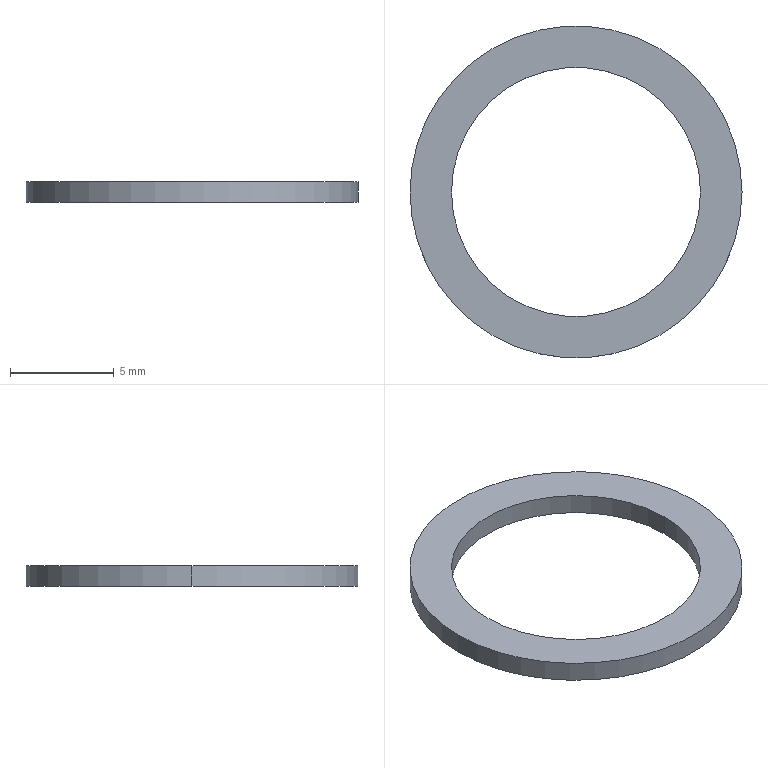Part | SolidWorks | features Extrusion 1 | 1 solid | 6 faces | box 16 x 16 x 1 mm | volume 87.965 mm3 | cylinder 4 | plane 2 | commonest cylinder face diameters 12 x2 16 x2
STEP:
#1=CARTESIAN_POINT('',(-6.,0.,1.));
#2=VERTEX_POINT('',#1);
#3=CARTESIAN_POINT('',(6.,0.,1.));
#4=VERTEX_POINT('',#3);
#5=CARTESIAN_POINT('',(0.,0.,1.));
#6=DIRECTION('',(0.,0.,1.));
#7=DIRECTION('',(1.,0.,0.));
#8=AXIS2_PLACEMENT_3D('',#5,#6,#7);
#9=CIRCLE('',#8,6.);
#10=EDGE_CURVE('',#2,#4,#9,.T.);
#11=ORIENTED_EDGE('',*,*,#10,.T.);
#12=CARTESIAN_POINT('',(6.,0.,0.));
#13=VERTEX_POINT('',#12);
#14=CARTESIAN_POINT('',(6.,0.,1.));
#15=DIRECTION('',(0.,0.,-1.));
#16=VECTOR('',#15,1000.);
#17=LINE('',#14,#16);
#18=EDGE_CURVE('',#4,#13,#17,.T.);
#19=ORIENTED_EDGE('',*,*,#18,.T.);
#20=CARTESIAN_POINT('',(-6.,0.,0.));
#21=VERTEX_POINT('',#20);
#22=CARTESIAN_POINT('',(0.,0.,0.));
#23=DIRECTION('',(0.,0.,1.));
#24=DIRECTION('',(1.,0.,0.));
#25=AXIS2_PLACEMENT_3D('',#22,#23,#24);
#26=CIRCLE('',#25,6.);
#27=EDGE_CURVE('',#21,#13,#26,.T.);
#28=ORIENTED_EDGE('',*,*,#27,.F.);
#29=CARTESIAN_POINT('',(-6.,0.,1.));
#30=DIRECTION('',(0.,0.,-1.));
#31=VECTOR('',#30,1000.);
#32=LINE('',#29,#31);
#33=EDGE_CURVE('',#2,#21,#32,.T.);
#34=ORIENTED_EDGE('',*,*,#33,.F.);
#35=EDGE_LOOP('',(#11,#19,#28,#34));
#36=FACE_OUTER_BOUND('',#35,.T.);
#37=CARTESIAN_POINT('',(0.,0.,1.));
#38=DIRECTION('',(0.,0.,-1.));
#39=DIRECTION('',(-1.,0.,0.));
#40=AXIS2_PLACEMENT_3D('',#37,#38,#39);
#41=CYLINDRICAL_SURFACE('',#40,6.);
#42=ADVANCED_FACE('',(#36),#41,.F.);
#43=CARTESIAN_POINT('',(8.,0.,1.));
#44=VERTEX_POINT('',#43);
#45=CARTESIAN_POINT('',(-8.,0.,1.));
#46=VERTEX_POINT('',#45);
#47=CARTESIAN_POINT('',(0.,0.,1.));
#48=DIRECTION('',(0.,0.,1.));
#49=DIRECTION('',(1.,0.,0.));
#50=AXIS2_PLACEMENT_3D('',#47,#48,#49);
#51=CIRCLE('',#50,8.);
#52=EDGE_CURVE('',#44,#46,#51,.T.);
#53=ORIENTED_EDGE('',*,*,#52,.F.);
#54=CARTESIAN_POINT('',(8.,0.,0.));
#55=VERTEX_POINT('',#54);
#56=CARTESIAN_POINT('',(8.,0.,1.));
#57=DIRECTION('',(0.,0.,-1.));
#58=VECTOR('',#57,1000.);
#59=LINE('',#56,#58);
#60=EDGE_CURVE('',#44,#55,#59,.T.);
#61=ORIENTED_EDGE('',*,*,#60,.T.);
#62=CARTESIAN_POINT('',(-8.,0.,0.));
#63=VERTEX_POINT('',#62);
#64=CARTESIAN_POINT('',(0.,0.,0.));
#65=DIRECTION('',(0.,0.,1.));
#66=DIRECTION('',(1.,0.,0.));
#67=AXIS2_PLACEMENT_3D('',#64,#65,#66);
#68=CIRCLE('',#67,8.);
#69=EDGE_CURVE('',#55,#63,#68,.T.);
#70=ORIENTED_EDGE('',*,*,#69,.T.);
#71=CARTESIAN_POINT('',(-8.,0.,1.));
#72=DIRECTION('',(0.,0.,-1.));
#73=VECTOR('',#72,1000.);
#74=LINE('',#71,#73);
#75=EDGE_CURVE('',#46,#63,#74,.T.);
#76=ORIENTED_EDGE('',*,*,#75,.F.);
#77=EDGE_LOOP('',(#53,#61,#70,#76));
#78=FACE_OUTER_BOUND('',#77,.T.);
#79=CARTESIAN_POINT('',(0.,0.,1.));
#80=DIRECTION('',(0.,0.,-1.));
#81=DIRECTION('',(-1.,0.,0.));
#82=AXIS2_PLACEMENT_3D('',#79,#80,#81);
#83=CYLINDRICAL_SURFACE('',#82,8.);
#84=ADVANCED_FACE('',(#78),#83,.T.);
#85=CARTESIAN_POINT('',(0.,0.,1.));
#86=DIRECTION('',(0.,0.,1.));
#87=DIRECTION('',(1.,0.,0.));
#88=AXIS2_PLACEMENT_3D('',#85,#86,#87);
#89=CIRCLE('',#88,8.);
#90=EDGE_CURVE('',#46,#44,#89,.T.);
#91=ORIENTED_EDGE('',*,*,#90,.T.);
#92=ORIENTED_EDGE('',*,*,#52,.T.);
#93=EDGE_LOOP('',(#91,#92));
#94=FACE_OUTER_BOUND('',#93,.T.);
#95=ORIENTED_EDGE('',*,*,#10,.F.);
#96=CARTESIAN_POINT('',(0.,0.,1.));
#97=DIRECTION('',(0.,0.,1.));
#98=DIRECTION('',(1.,0.,0.));
#99=AXIS2_PLACEMENT_3D('',#96,#97,#98);
#100=CIRCLE('',#99,6.);
#101=EDGE_CURVE('',#4,#2,#100,.T.);
#102=ORIENTED_EDGE('',*,*,#101,.F.);
#103=EDGE_LOOP('',(#95,#102));
#104=FACE_BOUND('',#103,.T.);
#105=CARTESIAN_POINT('',(0.,0.,1.));
#106=DIRECTION('',(0.,0.,1.));
#107=DIRECTION('',(1.,0.,0.));
#108=AXIS2_PLACEMENT_3D('',#105,#106,#107);
#109=PLANE('',#108);
#110=ADVANCED_FACE('',(#94,#104),#109,.T.);
#111=CARTESIAN_POINT('',(0.,0.,0.));
#112=DIRECTION('',(0.,0.,1.));
#113=DIRECTION('',(1.,0.,0.));
#114=AXIS2_PLACEMENT_3D('',#111,#112,#113);
#115=CIRCLE('',#114,8.);
#116=EDGE_CURVE('',#63,#55,#115,.T.);
#117=ORIENTED_EDGE('',*,*,#116,.F.);
#118=ORIENTED_EDGE('',*,*,#69,.F.);
#119=EDGE_LOOP('',(#117,#118));
#120=FACE_OUTER_BOUND('',#119,.T.);
#121=ORIENTED_EDGE('',*,*,#27,.T.);
#122=CARTESIAN_POINT('',(0.,0.,0.));
#123=DIRECTION('',(0.,0.,1.));
#124=DIRECTION('',(1.,0.,0.));
#125=AXIS2_PLACEMENT_3D('',#122,#123,#124);
#126=CIRCLE('',#125,6.);
#127=EDGE_CURVE('',#13,#21,#126,.T.);
#128=ORIENTED_EDGE('',*,*,#127,.T.);
#129=EDGE_LOOP('',(#121,#128));
#130=FACE_BOUND('',#129,.T.);
#131=CARTESIAN_POINT('',(0.,0.,0.));
#132=DIRECTION('',(0.,0.,1.));
#133=DIRECTION('',(1.,0.,0.));
#134=AXIS2_PLACEMENT_3D('',#131,#132,#133);
#135=PLANE('',#134);
#136=ADVANCED_FACE('',(#120,#130),#135,.F.);
#137=ORIENTED_EDGE('',*,*,#60,.F.);
#138=ORIENTED_EDGE('',*,*,#90,.F.);
#139=ORIENTED_EDGE('',*,*,#75,.T.);
#140=ORIENTED_EDGE('',*,*,#116,.T.);
#141=EDGE_LOOP('',(#137,#138,#139,#140));
#142=FACE_OUTER_BOUND('',#141,.T.);
#143=CARTESIAN_POINT('',(0.,0.,1.));
#144=DIRECTION('',(0.,0.,-1.));
#145=DIRECTION('',(-1.,0.,0.));
#146=AXIS2_PLACEMENT_3D('',#143,#144,#145);
#147=CYLINDRICAL_SURFACE('',#146,8.);
#148=ADVANCED_FACE('',(#142),#147,.T.);
#149=ORIENTED_EDGE('',*,*,#18,.F.);
#150=ORIENTED_EDGE('',*,*,#101,.T.);
#151=ORIENTED_EDGE('',*,*,#33,.T.);
#152=ORIENTED_EDGE('',*,*,#127,.F.);
#153=EDGE_LOOP('',(#149,#150,#151,#152));
#154=FACE_OUTER_BOUND('',#153,.T.);
#155=CARTESIAN_POINT('',(0.,0.,1.));
#156=DIRECTION('',(0.,0.,-1.));
#157=DIRECTION('',(-1.,0.,0.));
#158=AXIS2_PLACEMENT_3D('',#155,#156,#157);
#159=CYLINDRICAL_SURFACE('',#158,6.);
#160=ADVANCED_FACE('',(#154),#159,.F.);
#161=CLOSED_SHELL('',(#42,#84,#110,#136,#148,#160));
#162=MANIFOLD_SOLID_BREP('',#161);
#163=CARTESIAN_POINT('',(0.,0.,0.));
#164=DIRECTION('',(0.,0.,1.));
#165=DIRECTION('',(1.,0.,0.));
#166=AXIS2_PLACEMENT_3D('',#163,#164,#165);
#167=(LENGTH_UNIT()NAMED_UNIT(*)SI_UNIT(.MILLI.,.METRE.));
#168=UNCERTAINTY_MEASURE_WITH_UNIT(LENGTH_MEASURE(0.00001),#167,'','');
#169=(NAMED_UNIT(*)PLANE_ANGLE_UNIT()SI_UNIT($,.RADIAN.));
#170=(NAMED_UNIT(*)SI_UNIT($,.STERADIAN.)SOLID_ANGLE_UNIT());
#171=(GEOMETRIC_REPRESENTATION_CONTEXT(3)GLOBAL_UNCERTAINTY_ASSIGNED_CONTEXT((#168))GLOBAL_UNIT_ASSIGNED_CONTEXT((#167,#169,#170))REPRESENTATION_CONTEXT('',''));
#172=ADVANCED_BREP_SHAPE_REPRESENTATION('',(#162,#166),#171);